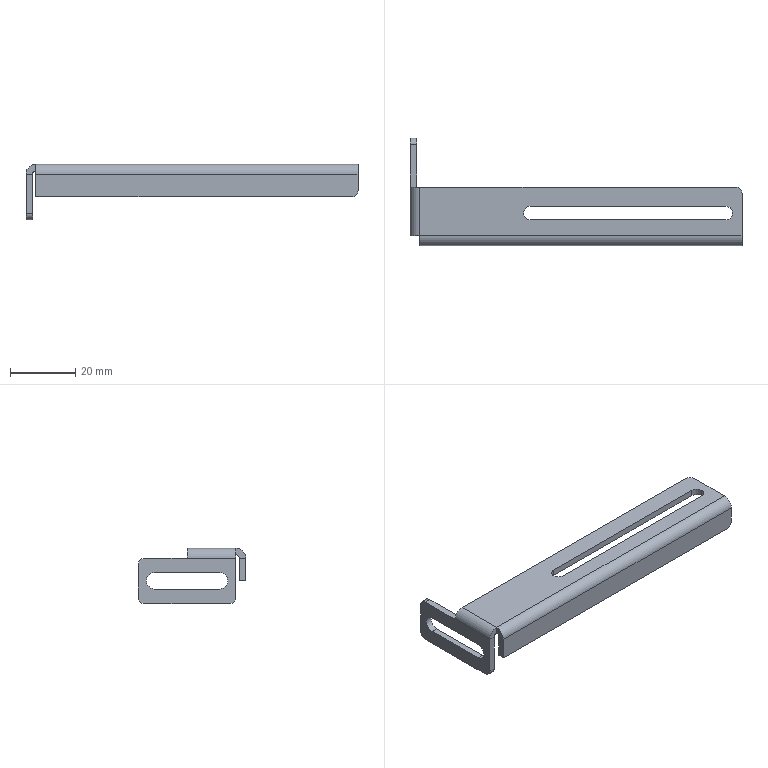Part | STEP file | ND25021-01-JDKM-03-BJ | 1 solid | 36 faces | box 102 x 33 x 17 mm | volume 5133 mm3 | plane 22 | cylinder 14 | commonest cylinder face diameters 4 x5 4.2 x3 2 x2 5 x2 6 x2